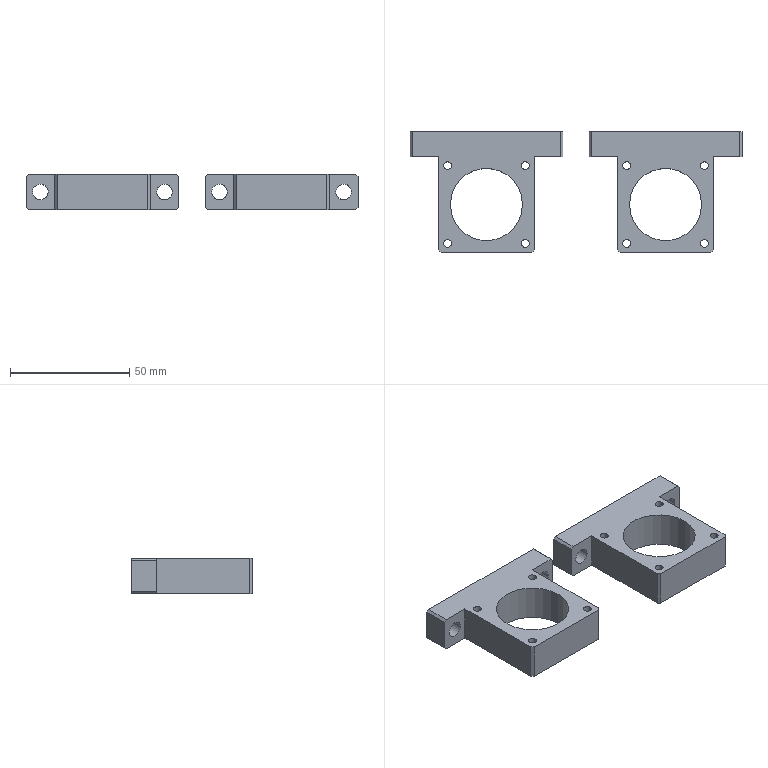Part | 2 solids | 46 faces | box 139 x 50.5 x 15 mm | volume 44135 mm3 | plane 32 | cylinder 14 | commonest cylinder face diameters 3.3 x8 6.6 x4 30.2 x2
STEP:
#1=CARTESIAN_POINT('',(94.,-25.25,7.5));
#2=VERTEX_POINT('',#1);
#3=CARTESIAN_POINT('',(95.,-24.25,7.5));
#4=VERTEX_POINT('',#3);
#5=CARTESIAN_POINT('',(95.,-24.25,7.5));
#6=DIRECTION('',(0.7071,0.7071,0.));
#7=VECTOR('',#6,1000.);
#8=LINE('',#5,#7);
#9=EDGE_CURVE('',#2,#4,#8,.T.);
#10=ORIENTED_EDGE('',*,*,#9,.F.);
#11=CARTESIAN_POINT('',(94.,-25.25,-7.5));
#12=VERTEX_POINT('',#11);
#13=CARTESIAN_POINT('',(94.,-25.25,7.5));
#14=DIRECTION('',(0.,0.,1.));
#15=VECTOR('',#14,1000.);
#16=LINE('',#13,#15);
#17=EDGE_CURVE('',#12,#2,#16,.T.);
#18=ORIENTED_EDGE('',*,*,#17,.F.);
#19=CARTESIAN_POINT('',(95.,-24.25,-7.5));
#20=VERTEX_POINT('',#19);
#21=CARTESIAN_POINT('',(97.125,-22.125,-7.5));
#22=DIRECTION('',(-0.7071,-0.7071,0.));
#23=VECTOR('',#22,1000.);
#24=LINE('',#21,#23);
#25=EDGE_CURVE('',#20,#12,#24,.T.);
#26=ORIENTED_EDGE('',*,*,#25,.F.);
#27=CARTESIAN_POINT('',(95.,-24.25,-7.5));
#28=DIRECTION('',(0.,0.,-1.));
#29=VECTOR('',#28,1000.);
#30=LINE('',#27,#29);
#31=EDGE_CURVE('',#4,#20,#30,.T.);
#32=ORIENTED_EDGE('',*,*,#31,.F.);
#33=EDGE_LOOP('',(#10,#18,#26,#32));
#34=FACE_BOUND('',#33,.T.);
#35=CARTESIAN_POINT('',(95.,-24.25,7.5));
#36=DIRECTION('',(0.7071,-0.7071,0.));
#37=DIRECTION('',(0.,0.,1.));
#38=AXIS2_PLACEMENT_3D('',#35,#36,#37);
#39=PLANE('',#38);
#40=ADVANCED_FACE('',(#34),#39,.T.);
#41=CARTESIAN_POINT('',(55.,-24.25,7.5));
#42=VERTEX_POINT('',#41);
#43=CARTESIAN_POINT('',(56.,-25.25,7.5));
#44=VERTEX_POINT('',#43);
#45=CARTESIAN_POINT('',(56.,-25.25,7.5));
#46=DIRECTION('',(0.7071,-0.7071,0.));
#47=VECTOR('',#46,1000.);
#48=LINE('',#45,#47);
#49=EDGE_CURVE('',#42,#44,#48,.T.);
#50=ORIENTED_EDGE('',*,*,#49,.F.);
#51=CARTESIAN_POINT('',(55.,-24.25,-7.5));
#52=VERTEX_POINT('',#51);
#53=CARTESIAN_POINT('',(55.,-24.25,7.5));
#54=DIRECTION('',(0.,0.,1.));
#55=VECTOR('',#54,1000.);
#56=LINE('',#53,#55);
#57=EDGE_CURVE('',#52,#42,#56,.T.);
#58=ORIENTED_EDGE('',*,*,#57,.F.);
#59=CARTESIAN_POINT('',(56.,-25.25,-7.5));
#60=VERTEX_POINT('',#59);
#61=CARTESIAN_POINT('',(52.875,-22.125,-7.5));
#62=DIRECTION('',(-0.7071,0.7071,0.));
#63=VECTOR('',#62,1000.);
#64=LINE('',#61,#63);
#65=EDGE_CURVE('',#60,#52,#64,.T.);
#66=ORIENTED_EDGE('',*,*,#65,.F.);
#67=CARTESIAN_POINT('',(56.,-25.25,-7.5));
#68=DIRECTION('',(0.,0.,-1.));
#69=VECTOR('',#68,1000.);
#70=LINE('',#67,#69);
#71=EDGE_CURVE('',#44,#60,#70,.T.);
#72=ORIENTED_EDGE('',*,*,#71,.F.);
#73=EDGE_LOOP('',(#50,#58,#66,#72));
#74=FACE_BOUND('',#73,.T.);
#75=CARTESIAN_POINT('',(56.,-25.25,7.5));
#76=DIRECTION('',(-0.7071,-0.7071,0.));
#77=DIRECTION('',(0.,0.,1.));
#78=AXIS2_PLACEMENT_3D('',#75,#76,#77);
#79=PLANE('',#78);
#80=ADVANCED_FACE('',(#74),#79,.T.);
#81=CARTESIAN_POINT('',(44.,14.75,7.5));
#82=VERTEX_POINT('',#81);
#83=CARTESIAN_POINT('',(43.,14.75,6.5));
#84=VERTEX_POINT('',#83);
#85=CARTESIAN_POINT('',(43.5,14.75,7.));
#86=DIRECTION('',(-0.7071,0.,-0.7071));
#87=VECTOR('',#86,1000.);
#88=LINE('',#85,#87);
#89=EDGE_CURVE('',#82,#84,#88,.T.);
#90=ORIENTED_EDGE('',*,*,#89,.F.);
#91=CARTESIAN_POINT('',(44.,25.25,7.5));
#92=VERTEX_POINT('',#91);
#93=CARTESIAN_POINT('',(44.,14.75,7.5));
#94=DIRECTION('',(0.,-1.,0.));
#95=VECTOR('',#94,1000.);
#96=LINE('',#93,#95);
#97=EDGE_CURVE('',#92,#82,#96,.T.);
#98=ORIENTED_EDGE('',*,*,#97,.F.);
#99=CARTESIAN_POINT('',(43.,25.25,6.5));
#100=VERTEX_POINT('',#99);
#101=CARTESIAN_POINT('',(43.5,25.25,7.));
#102=DIRECTION('',(0.7071,0.,0.7071));
#103=VECTOR('',#102,1000.);
#104=LINE('',#101,#103);
#105=EDGE_CURVE('',#100,#92,#104,.T.);
#106=ORIENTED_EDGE('',*,*,#105,.F.);
#107=CARTESIAN_POINT('',(43.,25.25,6.5));
#108=DIRECTION('',(0.,1.,0.));
#109=VECTOR('',#108,1000.);
#110=LINE('',#107,#109);
#111=EDGE_CURVE('',#84,#100,#110,.T.);
#112=ORIENTED_EDGE('',*,*,#111,.F.);
#113=EDGE_LOOP('',(#90,#98,#106,#112));
#114=FACE_BOUND('',#113,.T.);
#115=CARTESIAN_POINT('',(43.,-25.25,6.5));
#116=DIRECTION('',(-0.7071,0.,0.7071));
#117=DIRECTION('',(0.,-1.,0.));
#118=AXIS2_PLACEMENT_3D('',#115,#116,#117);
#119=PLANE('',#118);
#120=ADVANCED_FACE('',(#114),#119,.T.);
#121=CARTESIAN_POINT('',(43.,14.75,-6.5));
#122=VERTEX_POINT('',#121);
#123=CARTESIAN_POINT('',(44.,14.75,-7.5));
#124=VERTEX_POINT('',#123);
#125=CARTESIAN_POINT('',(36.,14.75,0.5));
#126=DIRECTION('',(0.7071,0.,-0.7071));
#127=VECTOR('',#126,1000.);
#128=LINE('',#125,#127);
#129=EDGE_CURVE('',#122,#124,#128,.T.);
#130=ORIENTED_EDGE('',*,*,#129,.F.);
#131=CARTESIAN_POINT('',(43.,25.25,-6.5));
#132=VERTEX_POINT('',#131);
#133=CARTESIAN_POINT('',(43.,-25.25,-6.5));
#134=DIRECTION('',(0.,-1.,0.));
#135=VECTOR('',#134,1000.);
#136=LINE('',#133,#135);
#137=EDGE_CURVE('',#132,#122,#136,.T.);
#138=ORIENTED_EDGE('',*,*,#137,.F.);
#139=CARTESIAN_POINT('',(44.,25.25,-7.5));
#140=VERTEX_POINT('',#139);
#141=CARTESIAN_POINT('',(36.,25.25,0.5));
#142=DIRECTION('',(-0.7071,0.,0.7071));
#143=VECTOR('',#142,1000.);
#144=LINE('',#141,#143);
#145=EDGE_CURVE('',#140,#132,#144,.T.);
#146=ORIENTED_EDGE('',*,*,#145,.F.);
#147=CARTESIAN_POINT('',(44.,0.,-7.5));
#148=DIRECTION('',(0.,1.,0.));
#149=VECTOR('',#148,1000.);
#150=LINE('',#147,#149);
#151=EDGE_CURVE('',#124,#140,#150,.T.);
#152=ORIENTED_EDGE('',*,*,#151,.F.);
#153=EDGE_LOOP('',(#130,#138,#146,#152));
#154=FACE_BOUND('',#153,.T.);
#155=CARTESIAN_POINT('',(44.,0.,-7.5));
#156=DIRECTION('',(0.7071,0.,0.7071));
#157=DIRECTION('',(0.,1.,0.));
#158=AXIS2_PLACEMENT_3D('',#155,#156,#157);
#159=PLANE('',#158);
#160=ADVANCED_FACE('',(#154),#159,.F.);
#161=CARTESIAN_POINT('',(107.,14.75,6.5));
#162=VERTEX_POINT('',#161);
#163=CARTESIAN_POINT('',(106.,14.75,7.5));
#164=VERTEX_POINT('',#163);
#165=CARTESIAN_POINT('',(74.5,14.75,39.));
#166=DIRECTION('',(-0.7071,0.,0.7071));
#167=VECTOR('',#166,1000.);
#168=LINE('',#165,#167);
#169=EDGE_CURVE('',#162,#164,#168,.T.);
#170=ORIENTED_EDGE('',*,*,#169,.F.);
#171=CARTESIAN_POINT('',(107.,25.25,6.5));
#172=VERTEX_POINT('',#171);
#173=CARTESIAN_POINT('',(107.,-25.25,6.5));
#174=DIRECTION('',(0.,-1.,0.));
#175=VECTOR('',#174,1000.);
#176=LINE('',#173,#175);
#177=EDGE_CURVE('',#172,#162,#176,.T.);
#178=ORIENTED_EDGE('',*,*,#177,.F.);
#179=CARTESIAN_POINT('',(106.,25.25,7.5));
#180=VERTEX_POINT('',#179);
#181=CARTESIAN_POINT('',(74.5,25.25,39.));
#182=DIRECTION('',(0.7071,0.,-0.7071));
#183=VECTOR('',#182,1000.);
#184=LINE('',#181,#183);
#185=EDGE_CURVE('',#180,#172,#184,.T.);
#186=ORIENTED_EDGE('',*,*,#185,.F.);
#187=CARTESIAN_POINT('',(106.,0.,7.5));
#188=DIRECTION('',(0.,1.,0.));
#189=VECTOR('',#188,1000.);
#190=LINE('',#187,#189);
#191=EDGE_CURVE('',#164,#180,#190,.T.);
#192=ORIENTED_EDGE('',*,*,#191,.F.);
#193=EDGE_LOOP('',(#170,#178,#186,#192));
#194=FACE_BOUND('',#193,.T.);
#195=CARTESIAN_POINT('',(106.,0.,7.5));
#196=DIRECTION('',(-0.7071,0.,-0.7071));
#197=DIRECTION('',(0.,1.,0.));
#198=AXIS2_PLACEMENT_3D('',#195,#196,#197);
#199=PLANE('',#198);
#200=ADVANCED_FACE('',(#194),#199,.F.);
#201=CARTESIAN_POINT('',(106.,14.75,-7.5));
#202=VERTEX_POINT('',#201);
#203=CARTESIAN_POINT('',(107.,14.75,-6.5));
#204=VERTEX_POINT('',#203);
#205=CARTESIAN_POINT('',(82.,14.75,-31.5));
#206=DIRECTION('',(0.7071,0.,0.7071));
#207=VECTOR('',#206,1000.);
#208=LINE('',#205,#207);
#209=EDGE_CURVE('',#202,#204,#208,.T.);
#210=ORIENTED_EDGE('',*,*,#209,.F.);
#211=CARTESIAN_POINT('',(106.,25.25,-7.5));
#212=VERTEX_POINT('',#211);
#213=CARTESIAN_POINT('',(106.,14.75,-7.5));
#214=DIRECTION('',(0.,-1.,0.));
#215=VECTOR('',#214,1000.);
#216=LINE('',#213,#215);
#217=EDGE_CURVE('',#212,#202,#216,.T.);
#218=ORIENTED_EDGE('',*,*,#217,.F.);
#219=CARTESIAN_POINT('',(107.,25.25,-6.5));
#220=VERTEX_POINT('',#219);
#221=CARTESIAN_POINT('',(82.,25.25,-31.5));
#222=DIRECTION('',(-0.7071,0.,-0.7071));
#223=VECTOR('',#222,1000.);
#224=LINE('',#221,#223);
#225=EDGE_CURVE('',#220,#212,#224,.T.);
#226=ORIENTED_EDGE('',*,*,#225,.F.);
#227=CARTESIAN_POINT('',(107.,25.25,-6.5));
#228=DIRECTION('',(0.,1.,0.));
#229=VECTOR('',#228,1000.);
#230=LINE('',#227,#229);
#231=EDGE_CURVE('',#204,#220,#230,.T.);
#232=ORIENTED_EDGE('',*,*,#231,.F.);
#233=EDGE_LOOP('',(#210,#218,#226,#232));
#234=FACE_BOUND('',#233,.T.);
#235=CARTESIAN_POINT('',(107.,-25.25,-6.5));
#236=DIRECTION('',(0.7071,0.,-0.7071));
#237=DIRECTION('',(0.,-1.,0.));
#238=AXIS2_PLACEMENT_3D('',#235,#236,#237);
#239=PLANE('',#238);
#240=ADVANCED_FACE('',(#234),#239,.T.);
#241=CARTESIAN_POINT('',(43.,14.75,7.5));
#242=DIRECTION('',(0.,0.,-1.));
#243=VECTOR('',#242,1000.);
#244=LINE('',#241,#243);
#245=EDGE_CURVE('',#84,#122,#244,.T.);
#246=ORIENTED_EDGE('',*,*,#245,.T.);
#247=ORIENTED_EDGE('',*,*,#129,.T.);
#248=CARTESIAN_POINT('',(55.,14.75,-7.5));
#249=VERTEX_POINT('',#248);
#250=CARTESIAN_POINT('',(43.,14.75,-7.5));
#251=DIRECTION('',(-1.,0.,0.));
#252=VECTOR('',#251,1000.);
#253=LINE('',#250,#252);
#254=EDGE_CURVE('',#249,#124,#253,.T.);
#255=ORIENTED_EDGE('',*,*,#254,.F.);
#256=CARTESIAN_POINT('',(55.,14.75,7.5));
#257=VERTEX_POINT('',#256);
#258=CARTESIAN_POINT('',(55.,14.75,7.5));
#259=DIRECTION('',(0.,0.,-1.));
#260=VECTOR('',#259,1000.);
#261=LINE('',#258,#260);
#262=EDGE_CURVE('',#257,#249,#261,.T.);
#263=ORIENTED_EDGE('',*,*,#262,.F.);
#264=CARTESIAN_POINT('',(43.,14.75,7.5));
#265=DIRECTION('',(-1.,0.,0.));
#266=VECTOR('',#265,1000.);
#267=LINE('',#264,#266);
#268=EDGE_CURVE('',#257,#82,#267,.T.);
#269=ORIENTED_EDGE('',*,*,#268,.T.);
#270=ORIENTED_EDGE('',*,*,#89,.T.);
#271=EDGE_LOOP('',(#246,#247,#255,#263,#269,#270));
#272=FACE_BOUND('',#271,.T.);
#273=CARTESIAN_POINT('',(52.3,14.75,0.));
#274=VERTEX_POINT('',#273);
#275=CARTESIAN_POINT('',(49.,14.75,0.));
#276=DIRECTION('',(0.,-1.,0.));
#277=DIRECTION('',(1.,0.,0.));
#278=AXIS2_PLACEMENT_3D('',#275,#276,#277);
#279=CIRCLE('',#278,3.3);
#280=EDGE_CURVE('',#274,#274,#279,.T.);
#281=ORIENTED_EDGE('',*,*,#280,.F.);
#282=EDGE_LOOP('',(#281));
#283=FACE_BOUND('',#282,.T.);
#284=CARTESIAN_POINT('',(43.,14.75,7.5));
#285=DIRECTION('',(0.,-1.,0.));
#286=DIRECTION('',(1.,0.,0.));
#287=AXIS2_PLACEMENT_3D('',#284,#285,#286);
#288=PLANE('',#287);
#289=ADVANCED_FACE('',(#272,#283),#288,.T.);
#290=CARTESIAN_POINT('',(55.,-25.25,-7.5));
#291=DIRECTION('',(0.,1.,0.));
#292=VECTOR('',#291,1000.);
#293=LINE('',#290,#292);
#294=EDGE_CURVE('',#52,#249,#293,.T.);
#295=ORIENTED_EDGE('',*,*,#294,.F.);
#296=ORIENTED_EDGE('',*,*,#57,.T.);
#297=CARTESIAN_POINT('',(55.,-25.25,7.5));
#298=DIRECTION('',(0.,1.,0.));
#299=VECTOR('',#298,1000.);
#300=LINE('',#297,#299);
#301=EDGE_CURVE('',#42,#257,#300,.T.);
#302=ORIENTED_EDGE('',*,*,#301,.T.);
#303=ORIENTED_EDGE('',*,*,#262,.T.);
#304=EDGE_LOOP('',(#295,#296,#302,#303));
#305=FACE_BOUND('',#304,.T.);
#306=CARTESIAN_POINT('',(55.,-25.25,7.5));
#307=DIRECTION('',(-1.,0.,0.));
#308=DIRECTION('',(0.,-1.,0.));
#309=AXIS2_PLACEMENT_3D('',#306,#307,#308);
#310=PLANE('',#309);
#311=ADVANCED_FACE('',(#305),#310,.T.);
#312=CARTESIAN_POINT('',(95.,14.75,7.5));
#313=VERTEX_POINT('',#312);
#314=CARTESIAN_POINT('',(95.,-25.25,7.5));
#315=DIRECTION('',(0.,-1.,0.));
#316=VECTOR('',#315,1000.);
#317=LINE('',#314,#316);
#318=EDGE_CURVE('',#313,#4,#317,.T.);
#319=ORIENTED_EDGE('',*,*,#318,.T.);
#320=ORIENTED_EDGE('',*,*,#31,.T.);
#321=CARTESIAN_POINT('',(95.,14.75,-7.5));
#322=VERTEX_POINT('',#321);
#323=CARTESIAN_POINT('',(95.,-25.25,-7.5));
#324=DIRECTION('',(0.,-1.,0.));
#325=VECTOR('',#324,1000.);
#326=LINE('',#323,#325);
#327=EDGE_CURVE('',#322,#20,#326,.T.);
#328=ORIENTED_EDGE('',*,*,#327,.F.);
#329=CARTESIAN_POINT('',(95.,14.75,7.5));
#330=DIRECTION('',(0.,0.,-1.));
#331=VECTOR('',#330,1000.);
#332=LINE('',#329,#331);
#333=EDGE_CURVE('',#313,#322,#332,.T.);
#334=ORIENTED_EDGE('',*,*,#333,.F.);
#335=EDGE_LOOP('',(#319,#320,#328,#334));
#336=FACE_BOUND('',#335,.T.);
#337=CARTESIAN_POINT('',(95.,-25.25,7.5));
#338=DIRECTION('',(1.,0.,0.));
#339=DIRECTION('',(0.,1.,0.));
#340=AXIS2_PLACEMENT_3D('',#337,#338,#339);
#341=PLANE('',#340);
#342=ADVANCED_FACE('',(#336),#341,.T.);
#343=CARTESIAN_POINT('',(75.,14.75,-7.5));
#344=DIRECTION('',(-1.,0.,0.));
#345=VECTOR('',#344,1000.);
#346=LINE('',#343,#345);
#347=EDGE_CURVE('',#202,#322,#346,.T.);
#348=ORIENTED_EDGE('',*,*,#347,.F.);
#349=ORIENTED_EDGE('',*,*,#209,.T.);
#350=CARTESIAN_POINT('',(107.,14.75,7.5));
#351=DIRECTION('',(0.,0.,-1.));
#352=VECTOR('',#351,1000.);
#353=LINE('',#350,#352);
#354=EDGE_CURVE('',#162,#204,#353,.T.);
#355=ORIENTED_EDGE('',*,*,#354,.F.);
#356=ORIENTED_EDGE('',*,*,#169,.T.);
#357=CARTESIAN_POINT('',(43.,14.75,7.5));
#358=DIRECTION('',(-1.,0.,0.));
#359=VECTOR('',#358,1000.);
#360=LINE('',#357,#359);
#361=EDGE_CURVE('',#164,#313,#360,.T.);
#362=ORIENTED_EDGE('',*,*,#361,.T.);
#363=ORIENTED_EDGE('',*,*,#333,.T.);
#364=EDGE_LOOP('',(#348,#349,#355,#356,#362,#363));
#365=FACE_BOUND('',#364,.T.);
#366=CARTESIAN_POINT('',(104.3,14.75,0.));
#367=VERTEX_POINT('',#366);
#368=CARTESIAN_POINT('',(101.,14.75,0.));
#369=DIRECTION('',(0.,-1.,0.));
#370=DIRECTION('',(1.,0.,0.));
#371=AXIS2_PLACEMENT_3D('',#368,#369,#370);
#372=CIRCLE('',#371,3.3);
#373=EDGE_CURVE('',#367,#367,#372,.T.);
#374=ORIENTED_EDGE('',*,*,#373,.F.);
#375=EDGE_LOOP('',(#374));
#376=FACE_BOUND('',#375,.T.);
#377=CARTESIAN_POINT('',(43.,14.75,7.5));
#378=DIRECTION('',(0.,-1.,0.));
#379=DIRECTION('',(1.,0.,0.));
#380=AXIS2_PLACEMENT_3D('',#377,#378,#379);
#381=PLANE('',#380);
#382=ADVANCED_FACE('',(#365,#376),#381,.T.);
#383=CARTESIAN_POINT('',(107.,25.25,7.5));
#384=DIRECTION('',(0.,0.,-1.));
#385=VECTOR('',#384,1000.);
#386=LINE('',#383,#385);
#387=EDGE_CURVE('',#172,#220,#386,.T.);
#388=ORIENTED_EDGE('',*,*,#387,.T.);
#389=ORIENTED_EDGE('',*,*,#225,.T.);
#390=CARTESIAN_POINT('',(43.,25.25,-7.5));
#391=DIRECTION('',(1.,0.,0.));
#392=VECTOR('',#391,1000.);
#393=LINE('',#390,#392);
#394=EDGE_CURVE('',#140,#212,#393,.T.);
#395=ORIENTED_EDGE('',*,*,#394,.F.);
#396=ORIENTED_EDGE('',*,*,#145,.T.);
#397=CARTESIAN_POINT('',(43.,25.25,7.5));
#398=DIRECTION('',(0.,0.,-1.));
#399=VECTOR('',#398,1000.);
#400=LINE('',#397,#399);
#401=EDGE_CURVE('',#100,#132,#400,.T.);
#402=ORIENTED_EDGE('',*,*,#401,.F.);
#403=ORIENTED_EDGE('',*,*,#105,.T.);
#404=CARTESIAN_POINT('',(43.,25.25,7.5));
#405=DIRECTION('',(1.,0.,0.));
#406=VECTOR('',#405,1000.);
#407=LINE('',#404,#406);
#408=EDGE_CURVE('',#92,#180,#407,.T.);
#409=ORIENTED_EDGE('',*,*,#408,.T.);
#410=ORIENTED_EDGE('',*,*,#185,.T.);
#411=EDGE_LOOP('',(#388,#389,#395,#396,#402,#403,#409,#410));
#412=FACE_BOUND('',#411,.T.);
#413=CARTESIAN_POINT('',(101.,25.25,3.3));
#414=VERTEX_POINT('',#413);
#415=CARTESIAN_POINT('',(101.,25.25,0.));
#416=DIRECTION('',(0.,1.,0.));
#417=DIRECTION('',(0.,0.,1.));
#418=AXIS2_PLACEMENT_3D('',#415,#416,#417);
#419=CIRCLE('',#418,3.3);
#420=EDGE_CURVE('',#414,#414,#419,.T.);
#421=ORIENTED_EDGE('',*,*,#420,.F.);
#422=EDGE_LOOP('',(#421));
#423=FACE_BOUND('',#422,.T.);
#424=CARTESIAN_POINT('',(49.,25.25,3.3));
#425=VERTEX_POINT('',#424);
#426=CARTESIAN_POINT('',(49.,25.25,0.));
#427=DIRECTION('',(0.,1.,0.));
#428=DIRECTION('',(0.,0.,1.));
#429=AXIS2_PLACEMENT_3D('',#426,#427,#428);
#430=CIRCLE('',#429,3.3);
#431=EDGE_CURVE('',#425,#425,#430,.T.);
#432=ORIENTED_EDGE('',*,*,#431,.F.);
#433=EDGE_LOOP('',(#432));
#434=FACE_BOUND('',#433,.T.);
#435=CARTESIAN_POINT('',(43.,25.25,7.5));
#436=DIRECTION('',(0.,1.,0.));
#437=DIRECTION('',(0.,0.,1.));
#438=AXIS2_PLACEMENT_3D('',#435,#436,#437);
#439=PLANE('',#438);
#440=ADVANCED_FACE('',(#412,#423,#434),#439,.T.);
#441=ORIENTED_EDGE('',*,*,#394,.T.);
#442=ORIENTED_EDGE('',*,*,#217,.T.);
#443=ORIENTED_EDGE('',*,*,#347,.T.);
#444=ORIENTED_EDGE('',*,*,#327,.T.);
#445=ORIENTED_EDGE('',*,*,#25,.T.);
#446=CARTESIAN_POINT('',(43.,-25.25,-7.5));
#447=DIRECTION('',(1.,0.,0.));
#448=VECTOR('',#447,1000.);
#449=LINE('',#446,#448);
#450=EDGE_CURVE('',#60,#12,#449,.T.);
#451=ORIENTED_EDGE('',*,*,#450,.F.);
#452=ORIENTED_EDGE('',*,*,#65,.T.);
#453=ORIENTED_EDGE('',*,*,#294,.T.);
#454=ORIENTED_EDGE('',*,*,#254,.T.);
#455=ORIENTED_EDGE('',*,*,#151,.T.);
#456=EDGE_LOOP('',(#441,#442,#443,#444,#445,#451,#452,#453,#454,#455));
#457=FACE_BOUND('',#456,.T.);
#458=CARTESIAN_POINT('',(59.9,-5.25,-7.5));
#459=VERTEX_POINT('',#458);
#460=CARTESIAN_POINT('',(75.,-5.25,-7.5));
#461=DIRECTION('',(0.,0.,-1.));
#462=DIRECTION('',(-1.,0.,0.));
#463=AXIS2_PLACEMENT_3D('',#460,#461,#462);
#464=CIRCLE('',#463,15.1);
#465=EDGE_CURVE('',#459,#459,#464,.T.);
#466=ORIENTED_EDGE('',*,*,#465,.F.);
#467=EDGE_LOOP('',(#466));
#468=FACE_BOUND('',#467,.T.);
#469=CARTESIAN_POINT('',(57.087,11.013,-7.5));
#470=VERTEX_POINT('',#469);
#471=CARTESIAN_POINT('',(58.737,11.013,-7.5));
#472=DIRECTION('',(0.,0.,-1.));
#473=DIRECTION('',(-1.,0.,0.));
#474=AXIS2_PLACEMENT_3D('',#471,#472,#473);
#475=CIRCLE('',#474,1.65);
#476=EDGE_CURVE('',#470,#470,#475,.T.);
#477=ORIENTED_EDGE('',*,*,#476,.F.);
#478=EDGE_LOOP('',(#477));
#479=FACE_BOUND('',#478,.T.);
#480=CARTESIAN_POINT('',(89.613,11.013,-7.5));
#481=VERTEX_POINT('',#480);
#482=CARTESIAN_POINT('',(91.263,11.013,-7.5));
#483=DIRECTION('',(0.,0.,-1.));
#484=DIRECTION('',(-1.,0.,0.));
#485=AXIS2_PLACEMENT_3D('',#482,#483,#484);
#486=CIRCLE('',#485,1.65);
#487=EDGE_CURVE('',#481,#481,#486,.T.);
#488=ORIENTED_EDGE('',*,*,#487,.F.);
#489=EDGE_LOOP('',(#488));
#490=FACE_BOUND('',#489,.T.);
#491=CARTESIAN_POINT('',(89.613,-21.513,-7.5));
#492=VERTEX_POINT('',#491);
#493=CARTESIAN_POINT('',(91.263,-21.513,-7.5));
#494=DIRECTION('',(0.,0.,-1.));
#495=DIRECTION('',(-1.,0.,0.));
#496=AXIS2_PLACEMENT_3D('',#493,#494,#495);
#497=CIRCLE('',#496,1.65);
#498=EDGE_CURVE('',#492,#492,#497,.T.);
#499=ORIENTED_EDGE('',*,*,#498,.F.);
#500=EDGE_LOOP('',(#499));
#501=FACE_BOUND('',#500,.T.);
#502=CARTESIAN_POINT('',(57.087,-21.513,-7.5));
#503=VERTEX_POINT('',#502);
#504=CARTESIAN_POINT('',(58.737,-21.513,-7.5));
#505=DIRECTION('',(0.,0.,-1.));
#506=DIRECTION('',(-1.,0.,0.));
#507=AXIS2_PLACEMENT_3D('',#504,#505,#506);
#508=CIRCLE('',#507,1.65);
#509=EDGE_CURVE('',#503,#503,#508,.T.);
#510=ORIENTED_EDGE('',*,*,#509,.F.);
#511=EDGE_LOOP('',(#510));
#512=FACE_BOUND('',#511,.T.);
#513=CARTESIAN_POINT('',(75.,0.,-7.5));
#514=DIRECTION('',(0.,0.,-1.));
#515=DIRECTION('',(-1.,0.,0.));
#516=AXIS2_PLACEMENT_3D('',#513,#514,#515);
#517=PLANE('',#516);
#518=ADVANCED_FACE('',(#457,#468,#479,#490,#501,#512),#517,.T.);
#519=ORIENTED_EDGE('',*,*,#361,.F.);
#520=ORIENTED_EDGE('',*,*,#191,.T.);
#521=ORIENTED_EDGE('',*,*,#408,.F.);
#522=ORIENTED_EDGE('',*,*,#97,.T.);
#523=ORIENTED_EDGE('',*,*,#268,.F.);
#524=ORIENTED_EDGE('',*,*,#301,.F.);
#525=ORIENTED_EDGE('',*,*,#49,.T.);
#526=CARTESIAN_POINT('',(43.,-25.25,7.5));
#527=DIRECTION('',(1.,0.,0.));
#528=VECTOR('',#527,1000.);
#529=LINE('',#526,#528);
#530=EDGE_CURVE('',#44,#2,#529,.T.);
#531=ORIENTED_EDGE('',*,*,#530,.T.);
#532=ORIENTED_EDGE('',*,*,#9,.T.);
#533=ORIENTED_EDGE('',*,*,#318,.F.);
#534=EDGE_LOOP('',(#519,#520,#521,#522,#523,#524,#525,#531,#532,#533));
#535=FACE_BOUND('',#534,.T.);
#536=CARTESIAN_POINT('',(59.9,-5.25,7.5));
#537=VERTEX_POINT('',#536);
#538=CARTESIAN_POINT('',(75.,-5.25,7.5));
#539=DIRECTION('',(0.,0.,-1.));
#540=DIRECTION('',(-1.,0.,0.));
#541=AXIS2_PLACEMENT_3D('',#538,#539,#540);
#542=CIRCLE('',#541,15.1);
#543=EDGE_CURVE('',#537,#537,#542,.T.);
#544=ORIENTED_EDGE('',*,*,#543,.T.);
#545=EDGE_LOOP('',(#544));
#546=FACE_BOUND('',#545,.T.);
#547=CARTESIAN_POINT('',(57.087,11.013,7.5));
#548=VERTEX_POINT('',#547);
#549=CARTESIAN_POINT('',(58.737,11.013,7.5));
#550=DIRECTION('',(0.,0.,-1.));
#551=DIRECTION('',(-1.,0.,0.));
#552=AXIS2_PLACEMENT_3D('',#549,#550,#551);
#553=CIRCLE('',#552,1.65);
#554=EDGE_CURVE('',#548,#548,#553,.T.);
#555=ORIENTED_EDGE('',*,*,#554,.T.);
#556=EDGE_LOOP('',(#555));
#557=FACE_BOUND('',#556,.T.);
#558=CARTESIAN_POINT('',(89.613,11.013,7.5));
#559=VERTEX_POINT('',#558);
#560=CARTESIAN_POINT('',(91.263,11.013,7.5));
#561=DIRECTION('',(0.,0.,-1.));
#562=DIRECTION('',(-1.,0.,0.));
#563=AXIS2_PLACEMENT_3D('',#560,#561,#562);
#564=CIRCLE('',#563,1.65);
#565=EDGE_CURVE('',#559,#559,#564,.T.);
#566=ORIENTED_EDGE('',*,*,#565,.T.);
#567=EDGE_LOOP('',(#566));
#568=FACE_BOUND('',#567,.T.);
#569=CARTESIAN_POINT('',(89.613,-21.513,7.5));
#570=VERTEX_POINT('',#569);
#571=CARTESIAN_POINT('',(91.263,-21.513,7.5));
#572=DIRECTION('',(0.,0.,-1.));
#573=DIRECTION('',(-1.,0.,0.));
#574=AXIS2_PLACEMENT_3D('',#571,#572,#573);
#575=CIRCLE('',#574,1.65);
#576=EDGE_CURVE('',#570,#570,#575,.T.);
#577=ORIENTED_EDGE('',*,*,#576,.T.);
#578=EDGE_LOOP('',(#577));
#579=FACE_BOUND('',#578,.T.);
#580=CARTESIAN_POINT('',(57.087,-21.513,7.5));
#581=VERTEX_POINT('',#580);
#582=CARTESIAN_POINT('',(58.737,-21.513,7.5));
#583=DIRECTION('',(0.,0.,-1.));
#584=DIRECTION('',(-1.,0.,0.));
#585=AXIS2_PLACEMENT_3D('',#582,#583,#584);
#586=CIRCLE('',#585,1.65);
#587=EDGE_CURVE('',#581,#581,#586,.T.);
#588=ORIENTED_EDGE('',*,*,#587,.T.);
#589=EDGE_LOOP('',(#588));
#590=FACE_BOUND('',#589,.T.);
#591=CARTESIAN_POINT('',(75.,0.,7.5));
#592=DIRECTION('',(0.,0.,-1.));
#593=DIRECTION('',(-1.,0.,0.));
#594=AXIS2_PLACEMENT_3D('',#591,#592,#593);
#595=PLANE('',#594);
#596=ADVANCED_FACE('',(#535,#546,#557,#568,#579,#590),#595,.F.);
#597=ORIENTED_EDGE('',*,*,#354,.T.);
#598=ORIENTED_EDGE('',*,*,#231,.T.);
#599=ORIENTED_EDGE('',*,*,#387,.F.);
#600=ORIENTED_EDGE('',*,*,#177,.T.);
#601=EDGE_LOOP('',(#597,#598,#599,#600));
#602=FACE_BOUND('',#601,.T.);
#603=CARTESIAN_POINT('',(107.,-25.25,7.5));
#604=DIRECTION('',(-1.,0.,0.));
#605=DIRECTION('',(0.,0.,1.));
#606=AXIS2_PLACEMENT_3D('',#603,#604,#605);
#607=PLANE('',#606);
#608=ADVANCED_FACE('',(#602),#607,.F.);
#609=ORIENTED_EDGE('',*,*,#530,.F.);
#610=ORIENTED_EDGE('',*,*,#71,.T.);
#611=ORIENTED_EDGE('',*,*,#450,.T.);
#612=ORIENTED_EDGE('',*,*,#17,.T.);
#613=EDGE_LOOP('',(#609,#610,#611,#612));
#614=FACE_BOUND('',#613,.T.);
#615=CARTESIAN_POINT('',(43.,-25.25,7.5));
#616=DIRECTION('',(0.,1.,0.));
#617=DIRECTION('',(0.,0.,1.));
#618=AXIS2_PLACEMENT_3D('',#615,#616,#617);
#619=PLANE('',#618);
#620=ADVANCED_FACE('',(#614),#619,.F.);
#621=ORIENTED_EDGE('',*,*,#401,.T.);
#622=ORIENTED_EDGE('',*,*,#137,.T.);
#623=ORIENTED_EDGE('',*,*,#245,.F.);
#624=ORIENTED_EDGE('',*,*,#111,.T.);
#625=EDGE_LOOP('',(#621,#622,#623,#624));
#626=FACE_BOUND('',#625,.T.);
#627=CARTESIAN_POINT('',(43.,-25.25,7.5));
#628=DIRECTION('',(-1.,0.,0.));
#629=DIRECTION('',(0.,0.,1.));
#630=AXIS2_PLACEMENT_3D('',#627,#628,#629);
#631=PLANE('',#630);
#632=ADVANCED_FACE('',(#626),#631,.T.);
#633=ORIENTED_EDGE('',*,*,#465,.T.);
#634=EDGE_LOOP('',(#633));
#635=FACE_BOUND('',#634,.T.);
#636=ORIENTED_EDGE('',*,*,#543,.F.);
#637=EDGE_LOOP('',(#636));
#638=FACE_BOUND('',#637,.T.);
#639=CARTESIAN_POINT('',(75.,-5.25,7.5));
#640=DIRECTION('',(0.,0.,-1.));
#641=DIRECTION('',(-1.,0.,0.));
#642=AXIS2_PLACEMENT_3D('',#639,#640,#641);
#643=CYLINDRICAL_SURFACE('',#642,15.1);
#644=ADVANCED_FACE('',(#635,#638),#643,.F.);
#645=ORIENTED_EDGE('',*,*,#476,.T.);
#646=EDGE_LOOP('',(#645));
#647=FACE_BOUND('',#646,.T.);
#648=ORIENTED_EDGE('',*,*,#554,.F.);
#649=EDGE_LOOP('',(#648));
#650=FACE_BOUND('',#649,.T.);
#651=CARTESIAN_POINT('',(58.737,11.013,-7.5));
#652=DIRECTION('',(0.,0.,-1.));
#653=DIRECTION('',(-1.,0.,0.));
#654=AXIS2_PLACEMENT_3D('',#651,#652,#653);
#655=CYLINDRICAL_SURFACE('',#654,1.65);
#656=ADVANCED_FACE('',(#647,#650),#655,.F.);
#657=ORIENTED_EDGE('',*,*,#487,.T.);
#658=EDGE_LOOP('',(#657));
#659=FACE_BOUND('',#658,.T.);
#660=ORIENTED_EDGE('',*,*,#565,.F.);
#661=EDGE_LOOP('',(#660));
#662=FACE_BOUND('',#661,.T.);
#663=CARTESIAN_POINT('',(91.263,11.013,-7.5));
#664=DIRECTION('',(0.,0.,-1.));
#665=DIRECTION('',(-1.,0.,0.));
#666=AXIS2_PLACEMENT_3D('',#663,#664,#665);
#667=CYLINDRICAL_SURFACE('',#666,1.65);
#668=ADVANCED_FACE('',(#659,#662),#667,.F.);
#669=ORIENTED_EDGE('',*,*,#498,.T.);
#670=EDGE_LOOP('',(#669));
#671=FACE_BOUND('',#670,.T.);
#672=ORIENTED_EDGE('',*,*,#576,.F.);
#673=EDGE_LOOP('',(#672));
#674=FACE_BOUND('',#673,.T.);
#675=CARTESIAN_POINT('',(91.263,-21.513,-7.5));
#676=DIRECTION('',(0.,0.,-1.));
#677=DIRECTION('',(-1.,0.,0.));
#678=AXIS2_PLACEMENT_3D('',#675,#676,#677);
#679=CYLINDRICAL_SURFACE('',#678,1.65);
#680=ADVANCED_FACE('',(#671,#674),#679,.F.);
#681=ORIENTED_EDGE('',*,*,#509,.T.);
#682=EDGE_LOOP('',(#681));
#683=FACE_BOUND('',#682,.T.);
#684=ORIENTED_EDGE('',*,*,#587,.F.);
#685=EDGE_LOOP('',(#684));
#686=FACE_BOUND('',#685,.T.);
#687=CARTESIAN_POINT('',(58.737,-21.513,-7.5));
#688=DIRECTION('',(0.,0.,-1.));
#689=DIRECTION('',(-1.,0.,0.));
#690=AXIS2_PLACEMENT_3D('',#687,#688,#689);
#691=CYLINDRICAL_SURFACE('',#690,1.65);
#692=ADVANCED_FACE('',(#683,#686),#691,.F.);
#693=ORIENTED_EDGE('',*,*,#373,.T.);
#694=EDGE_LOOP('',(#693));
#695=FACE_BOUND('',#694,.T.);
#696=ORIENTED_EDGE('',*,*,#420,.T.);
#697=EDGE_LOOP('',(#696));
#698=FACE_BOUND('',#697,.T.);
#699=CARTESIAN_POINT('',(101.,25.25,0.));
#700=DIRECTION('',(0.,1.,0.));
#701=DIRECTION('',(0.,0.,1.));
#702=AXIS2_PLACEMENT_3D('',#699,#700,#701);
#703=CYLINDRICAL_SURFACE('',#702,3.3);
#704=ADVANCED_FACE('',(#695,#698),#703,.F.);
#705=ORIENTED_EDGE('',*,*,#280,.T.);
#706=EDGE_LOOP('',(#705));
#707=FACE_BOUND('',#706,.T.);
#708=ORIENTED_EDGE('',*,*,#431,.T.);
#709=EDGE_LOOP('',(#708));
#710=FACE_BOUND('',#709,.T.);
#711=CARTESIAN_POINT('',(49.,25.25,0.));
#712=DIRECTION('',(0.,1.,0.));
#713=DIRECTION('',(0.,0.,1.));
#714=AXIS2_PLACEMENT_3D('',#711,#712,#713);
#715=CYLINDRICAL_SURFACE('',#714,3.3);
#716=ADVANCED_FACE('',(#707,#710),#715,.F.);
#717=CLOSED_SHELL('',(#40,#80,#120,#160,#200,#240,#289,#311,#342,#382,#440,#518,#596,#608,#620,#632,#644,#656,#668,#680,#692,#704,#716));
#718=MANIFOLD_SOLID_BREP('',#717);
#719=CARTESIAN_POINT('',(19.,-25.25,7.5));
#720=VERTEX_POINT('',#719);
#721=CARTESIAN_POINT('',(20.,-24.25,7.5));
#722=VERTEX_POINT('',#721);
#723=CARTESIAN_POINT('',(20.,-24.25,7.5));
#724=DIRECTION('',(0.7071,0.7071,0.));
#725=VECTOR('',#724,1000.);
#726=LINE('',#723,#725);
#727=EDGE_CURVE('',#720,#722,#726,.T.);
#728=ORIENTED_EDGE('',*,*,#727,.F.);
#729=CARTESIAN_POINT('',(19.,-25.25,-7.5));
#730=VERTEX_POINT('',#729);
#731=CARTESIAN_POINT('',(19.,-25.25,7.5));
#732=DIRECTION('',(0.,0.,1.));
#733=VECTOR('',#732,1000.);
#734=LINE('',#731,#733);
#735=EDGE_CURVE('',#730,#720,#734,.T.);
#736=ORIENTED_EDGE('',*,*,#735,.F.);
#737=CARTESIAN_POINT('',(20.,-24.25,-7.5));
#738=VERTEX_POINT('',#737);
#739=CARTESIAN_POINT('',(22.125,-22.125,-7.5));
#740=DIRECTION('',(-0.7071,-0.7071,0.));
#741=VECTOR('',#740,1000.);
#742=LINE('',#739,#741);
#743=EDGE_CURVE('',#738,#730,#742,.T.);
#744=ORIENTED_EDGE('',*,*,#743,.F.);
#745=CARTESIAN_POINT('',(20.,-24.25,-7.5));
#746=DIRECTION('',(0.,0.,-1.));
#747=VECTOR('',#746,1000.);
#748=LINE('',#745,#747);
#749=EDGE_CURVE('',#722,#738,#748,.T.);
#750=ORIENTED_EDGE('',*,*,#749,.F.);
#751=EDGE_LOOP('',(#728,#736,#744,#750));
#752=FACE_BOUND('',#751,.T.);
#753=CARTESIAN_POINT('',(20.,-24.25,7.5));
#754=DIRECTION('',(0.7071,-0.7071,0.));
#755=DIRECTION('',(0.,0.,1.));
#756=AXIS2_PLACEMENT_3D('',#753,#754,#755);
#757=PLANE('',#756);
#758=ADVANCED_FACE('',(#752),#757,.T.);
#759=CARTESIAN_POINT('',(-20.,-24.25,7.5));
#760=VERTEX_POINT('',#759);
#761=CARTESIAN_POINT('',(-19.,-25.25,7.5));
#762=VERTEX_POINT('',#761);
#763=CARTESIAN_POINT('',(-19.,-25.25,7.5));
#764=DIRECTION('',(0.7071,-0.7071,0.));
#765=VECTOR('',#764,1000.);
#766=LINE('',#763,#765);
#767=EDGE_CURVE('',#760,#762,#766,.T.);
#768=ORIENTED_EDGE('',*,*,#767,.F.);
#769=CARTESIAN_POINT('',(-20.,-24.25,-7.5));
#770=VERTEX_POINT('',#769);
#771=CARTESIAN_POINT('',(-20.,-24.25,7.5));
#772=DIRECTION('',(0.,0.,1.));
#773=VECTOR('',#772,1000.);
#774=LINE('',#771,#773);
#775=EDGE_CURVE('',#770,#760,#774,.T.);
#776=ORIENTED_EDGE('',*,*,#775,.F.);
#777=CARTESIAN_POINT('',(-19.,-25.25,-7.5));
#778=VERTEX_POINT('',#777);
#779=CARTESIAN_POINT('',(-22.125,-22.125,-7.5));
#780=DIRECTION('',(-0.7071,0.7071,0.));
#781=VECTOR('',#780,1000.);
#782=LINE('',#779,#781);
#783=EDGE_CURVE('',#778,#770,#782,.T.);
#784=ORIENTED_EDGE('',*,*,#783,.F.);
#785=CARTESIAN_POINT('',(-19.,-25.25,-7.5));
#786=DIRECTION('',(0.,0.,-1.));
#787=VECTOR('',#786,1000.);
#788=LINE('',#785,#787);
#789=EDGE_CURVE('',#762,#778,#788,.T.);
#790=ORIENTED_EDGE('',*,*,#789,.F.);
#791=EDGE_LOOP('',(#768,#776,#784,#790));
#792=FACE_BOUND('',#791,.T.);
#793=CARTESIAN_POINT('',(-19.,-25.25,7.5));
#794=DIRECTION('',(-0.7071,-0.7071,0.));
#795=DIRECTION('',(0.,0.,1.));
#796=AXIS2_PLACEMENT_3D('',#793,#794,#795);
#797=PLANE('',#796);
#798=ADVANCED_FACE('',(#792),#797,.T.);
#799=CARTESIAN_POINT('',(-31.,14.75,7.5));
#800=VERTEX_POINT('',#799);
#801=CARTESIAN_POINT('',(-32.,14.75,6.5));
#802=VERTEX_POINT('',#801);
#803=CARTESIAN_POINT('',(-31.5,14.75,7.));
#804=DIRECTION('',(-0.7071,0.,-0.7071));
#805=VECTOR('',#804,1000.);
#806=LINE('',#803,#805);
#807=EDGE_CURVE('',#800,#802,#806,.T.);
#808=ORIENTED_EDGE('',*,*,#807,.F.);
#809=CARTESIAN_POINT('',(-31.,25.25,7.5));
#810=VERTEX_POINT('',#809);
#811=CARTESIAN_POINT('',(-31.,14.75,7.5));
#812=DIRECTION('',(0.,-1.,0.));
#813=VECTOR('',#812,1000.);
#814=LINE('',#811,#813);
#815=EDGE_CURVE('',#810,#800,#814,.T.);
#816=ORIENTED_EDGE('',*,*,#815,.F.);
#817=CARTESIAN_POINT('',(-32.,25.25,6.5));
#818=VERTEX_POINT('',#817);
#819=CARTESIAN_POINT('',(-31.5,25.25,7.));
#820=DIRECTION('',(0.7071,0.,0.7071));
#821=VECTOR('',#820,1000.);
#822=LINE('',#819,#821);
#823=EDGE_CURVE('',#818,#810,#822,.T.);
#824=ORIENTED_EDGE('',*,*,#823,.F.);
#825=CARTESIAN_POINT('',(-32.,25.25,6.5));
#826=DIRECTION('',(0.,1.,0.));
#827=VECTOR('',#826,1000.);
#828=LINE('',#825,#827);
#829=EDGE_CURVE('',#802,#818,#828,.T.);
#830=ORIENTED_EDGE('',*,*,#829,.F.);
#831=EDGE_LOOP('',(#808,#816,#824,#830));
#832=FACE_BOUND('',#831,.T.);
#833=CARTESIAN_POINT('',(-32.,-25.25,6.5));
#834=DIRECTION('',(-0.7071,0.,0.7071));
#835=DIRECTION('',(0.,-1.,0.));
#836=AXIS2_PLACEMENT_3D('',#833,#834,#835);
#837=PLANE('',#836);
#838=ADVANCED_FACE('',(#832),#837,.T.);
#839=CARTESIAN_POINT('',(-32.,14.75,-6.5));
#840=VERTEX_POINT('',#839);
#841=CARTESIAN_POINT('',(-31.,14.75,-7.5));
#842=VERTEX_POINT('',#841);
#843=CARTESIAN_POINT('',(-39.,14.75,0.5));
#844=DIRECTION('',(0.7071,0.,-0.7071));
#845=VECTOR('',#844,1000.);
#846=LINE('',#843,#845);
#847=EDGE_CURVE('',#840,#842,#846,.T.);
#848=ORIENTED_EDGE('',*,*,#847,.F.);
#849=CARTESIAN_POINT('',(-32.,25.25,-6.5));
#850=VERTEX_POINT('',#849);
#851=CARTESIAN_POINT('',(-32.,-25.25,-6.5));
#852=DIRECTION('',(0.,-1.,0.));
#853=VECTOR('',#852,1000.);
#854=LINE('',#851,#853);
#855=EDGE_CURVE('',#850,#840,#854,.T.);
#856=ORIENTED_EDGE('',*,*,#855,.F.);
#857=CARTESIAN_POINT('',(-31.,25.25,-7.5));
#858=VERTEX_POINT('',#857);
#859=CARTESIAN_POINT('',(-39.,25.25,0.5));
#860=DIRECTION('',(-0.7071,0.,0.7071));
#861=VECTOR('',#860,1000.);
#862=LINE('',#859,#861);
#863=EDGE_CURVE('',#858,#850,#862,.T.);
#864=ORIENTED_EDGE('',*,*,#863,.F.);
#865=CARTESIAN_POINT('',(-31.,0.,-7.5));
#866=DIRECTION('',(0.,1.,0.));
#867=VECTOR('',#866,1000.);
#868=LINE('',#865,#867);
#869=EDGE_CURVE('',#842,#858,#868,.T.);
#870=ORIENTED_EDGE('',*,*,#869,.F.);
#871=EDGE_LOOP('',(#848,#856,#864,#870));
#872=FACE_BOUND('',#871,.T.);
#873=CARTESIAN_POINT('',(-31.,0.,-7.5));
#874=DIRECTION('',(0.7071,0.,0.7071));
#875=DIRECTION('',(0.,1.,0.));
#876=AXIS2_PLACEMENT_3D('',#873,#874,#875);
#877=PLANE('',#876);
#878=ADVANCED_FACE('',(#872),#877,.F.);
#879=CARTESIAN_POINT('',(32.,14.75,6.5));
#880=VERTEX_POINT('',#879);
#881=CARTESIAN_POINT('',(31.,14.75,7.5));
#882=VERTEX_POINT('',#881);
#883=CARTESIAN_POINT('',(-0.5,14.75,39.));
#884=DIRECTION('',(-0.7071,0.,0.7071));
#885=VECTOR('',#884,1000.);
#886=LINE('',#883,#885);
#887=EDGE_CURVE('',#880,#882,#886,.T.);
#888=ORIENTED_EDGE('',*,*,#887,.F.);
#889=CARTESIAN_POINT('',(32.,25.25,6.5));
#890=VERTEX_POINT('',#889);
#891=CARTESIAN_POINT('',(32.,-25.25,6.5));
#892=DIRECTION('',(0.,-1.,0.));
#893=VECTOR('',#892,1000.);
#894=LINE('',#891,#893);
#895=EDGE_CURVE('',#890,#880,#894,.T.);
#896=ORIENTED_EDGE('',*,*,#895,.F.);
#897=CARTESIAN_POINT('',(31.,25.25,7.5));
#898=VERTEX_POINT('',#897);
#899=CARTESIAN_POINT('',(-0.5,25.25,39.));
#900=DIRECTION('',(0.7071,0.,-0.7071));
#901=VECTOR('',#900,1000.);
#902=LINE('',#899,#901);
#903=EDGE_CURVE('',#898,#890,#902,.T.);
#904=ORIENTED_EDGE('',*,*,#903,.F.);
#905=CARTESIAN_POINT('',(31.,0.,7.5));
#906=DIRECTION('',(0.,1.,0.));
#907=VECTOR('',#906,1000.);
#908=LINE('',#905,#907);
#909=EDGE_CURVE('',#882,#898,#908,.T.);
#910=ORIENTED_EDGE('',*,*,#909,.F.);
#911=EDGE_LOOP('',(#888,#896,#904,#910));
#912=FACE_BOUND('',#911,.T.);
#913=CARTESIAN_POINT('',(31.,0.,7.5));
#914=DIRECTION('',(-0.7071,0.,-0.7071));
#915=DIRECTION('',(0.,1.,0.));
#916=AXIS2_PLACEMENT_3D('',#913,#914,#915);
#917=PLANE('',#916);
#918=ADVANCED_FACE('',(#912),#917,.F.);
#919=CARTESIAN_POINT('',(31.,14.75,-7.5));
#920=VERTEX_POINT('',#919);
#921=CARTESIAN_POINT('',(32.,14.75,-6.5));
#922=VERTEX_POINT('',#921);
#923=CARTESIAN_POINT('',(7.,14.75,-31.5));
#924=DIRECTION('',(0.7071,0.,0.7071));
#925=VECTOR('',#924,1000.);
#926=LINE('',#923,#925);
#927=EDGE_CURVE('',#920,#922,#926,.T.);
#928=ORIENTED_EDGE('',*,*,#927,.F.);
#929=CARTESIAN_POINT('',(31.,25.25,-7.5));
#930=VERTEX_POINT('',#929);
#931=CARTESIAN_POINT('',(31.,14.75,-7.5));
#932=DIRECTION('',(0.,-1.,0.));
#933=VECTOR('',#932,1000.);
#934=LINE('',#931,#933);
#935=EDGE_CURVE('',#930,#920,#934,.T.);
#936=ORIENTED_EDGE('',*,*,#935,.F.);
#937=CARTESIAN_POINT('',(32.,25.25,-6.5));
#938=VERTEX_POINT('',#937);
#939=CARTESIAN_POINT('',(7.,25.25,-31.5));
#940=DIRECTION('',(-0.7071,0.,-0.7071));
#941=VECTOR('',#940,1000.);
#942=LINE('',#939,#941);
#943=EDGE_CURVE('',#938,#930,#942,.T.);
#944=ORIENTED_EDGE('',*,*,#943,.F.);
#945=CARTESIAN_POINT('',(32.,25.25,-6.5));
#946=DIRECTION('',(0.,1.,0.));
#947=VECTOR('',#946,1000.);
#948=LINE('',#945,#947);
#949=EDGE_CURVE('',#922,#938,#948,.T.);
#950=ORIENTED_EDGE('',*,*,#949,.F.);
#951=EDGE_LOOP('',(#928,#936,#944,#950));
#952=FACE_BOUND('',#951,.T.);
#953=CARTESIAN_POINT('',(32.,-25.25,-6.5));
#954=DIRECTION('',(0.7071,0.,-0.7071));
#955=DIRECTION('',(0.,-1.,0.));
#956=AXIS2_PLACEMENT_3D('',#953,#954,#955);
#957=PLANE('',#956);
#958=ADVANCED_FACE('',(#952),#957,.T.);
#959=CARTESIAN_POINT('',(-32.,14.75,7.5));
#960=DIRECTION('',(0.,0.,-1.));
#961=VECTOR('',#960,1000.);
#962=LINE('',#959,#961);
#963=EDGE_CURVE('',#802,#840,#962,.T.);
#964=ORIENTED_EDGE('',*,*,#963,.T.);
#965=ORIENTED_EDGE('',*,*,#847,.T.);
#966=CARTESIAN_POINT('',(-20.,14.75,-7.5));
#967=VERTEX_POINT('',#966);
#968=CARTESIAN_POINT('',(-32.,14.75,-7.5));
#969=DIRECTION('',(-1.,0.,0.));
#970=VECTOR('',#969,1000.);
#971=LINE('',#968,#970);
#972=EDGE_CURVE('',#967,#842,#971,.T.);
#973=ORIENTED_EDGE('',*,*,#972,.F.);
#974=CARTESIAN_POINT('',(-20.,14.75,7.5));
#975=VERTEX_POINT('',#974);
#976=CARTESIAN_POINT('',(-20.,14.75,7.5));
#977=DIRECTION('',(0.,0.,-1.));
#978=VECTOR('',#977,1000.);
#979=LINE('',#976,#978);
#980=EDGE_CURVE('',#975,#967,#979,.T.);
#981=ORIENTED_EDGE('',*,*,#980,.F.);
#982=CARTESIAN_POINT('',(-32.,14.75,7.5));
#983=DIRECTION('',(-1.,0.,0.));
#984=VECTOR('',#983,1000.);
#985=LINE('',#982,#984);
#986=EDGE_CURVE('',#975,#800,#985,.T.);
#987=ORIENTED_EDGE('',*,*,#986,.T.);
#988=ORIENTED_EDGE('',*,*,#807,.T.);
#989=EDGE_LOOP('',(#964,#965,#973,#981,#987,#988));
#990=FACE_BOUND('',#989,.T.);
#991=CARTESIAN_POINT('',(-22.7,14.75,0.));
#992=VERTEX_POINT('',#991);
#993=CARTESIAN_POINT('',(-26.,14.75,0.));
#994=DIRECTION('',(0.,-1.,0.));
#995=DIRECTION('',(1.,0.,0.));
#996=AXIS2_PLACEMENT_3D('',#993,#994,#995);
#997=CIRCLE('',#996,3.3);
#998=EDGE_CURVE('',#992,#992,#997,.T.);
#999=ORIENTED_EDGE('',*,*,#998,.F.);
#1000=EDGE_LOOP('',(#999));
#1001=FACE_BOUND('',#1000,.T.);
#1002=CARTESIAN_POINT('',(-32.,14.75,7.5));
#1003=DIRECTION('',(0.,-1.,0.));
#1004=DIRECTION('',(1.,0.,0.));
#1005=AXIS2_PLACEMENT_3D('',#1002,#1003,#1004);
#1006=PLANE('',#1005);
#1007=ADVANCED_FACE('',(#990,#1001),#1006,.T.);
#1008=CARTESIAN_POINT('',(-20.,-25.25,-7.5));
#1009=DIRECTION('',(0.,1.,0.));
#1010=VECTOR('',#1009,1000.);
#1011=LINE('',#1008,#1010);
#1012=EDGE_CURVE('',#770,#967,#1011,.T.);
#1013=ORIENTED_EDGE('',*,*,#1012,.F.);
#1014=ORIENTED_EDGE('',*,*,#775,.T.);
#1015=CARTESIAN_POINT('',(-20.,-25.25,7.5));
#1016=DIRECTION('',(0.,1.,0.));
#1017=VECTOR('',#1016,1000.);
#1018=LINE('',#1015,#1017);
#1019=EDGE_CURVE('',#760,#975,#1018,.T.);
#1020=ORIENTED_EDGE('',*,*,#1019,.T.);
#1021=ORIENTED_EDGE('',*,*,#980,.T.);
#1022=EDGE_LOOP('',(#1013,#1014,#1020,#1021));
#1023=FACE_BOUND('',#1022,.T.);
#1024=CARTESIAN_POINT('',(-20.,-25.25,7.5));
#1025=DIRECTION('',(-1.,0.,0.));
#1026=DIRECTION('',(0.,-1.,0.));
#1027=AXIS2_PLACEMENT_3D('',#1024,#1025,#1026);
#1028=PLANE('',#1027);
#1029=ADVANCED_FACE('',(#1023),#1028,.T.);
#1030=CARTESIAN_POINT('',(20.,14.75,7.5));
#1031=VERTEX_POINT('',#1030);
#1032=CARTESIAN_POINT('',(20.,-25.25,7.5));
#1033=DIRECTION('',(0.,-1.,0.));
#1034=VECTOR('',#1033,1000.);
#1035=LINE('',#1032,#1034);
#1036=EDGE_CURVE('',#1031,#722,#1035,.T.);
#1037=ORIENTED_EDGE('',*,*,#1036,.T.);
#1038=ORIENTED_EDGE('',*,*,#749,.T.);
#1039=CARTESIAN_POINT('',(20.,14.75,-7.5));
#1040=VERTEX_POINT('',#1039);
#1041=CARTESIAN_POINT('',(20.,-25.25,-7.5));
#1042=DIRECTION('',(0.,-1.,0.));
#1043=VECTOR('',#1042,1000.);
#1044=LINE('',#1041,#1043);
#1045=EDGE_CURVE('',#1040,#738,#1044,.T.);
#1046=ORIENTED_EDGE('',*,*,#1045,.F.);
#1047=CARTESIAN_POINT('',(20.,14.75,7.5));
#1048=DIRECTION('',(0.,0.,-1.));
#1049=VECTOR('',#1048,1000.);
#1050=LINE('',#1047,#1049);
#1051=EDGE_CURVE('',#1031,#1040,#1050,.T.);
#1052=ORIENTED_EDGE('',*,*,#1051,.F.);
#1053=EDGE_LOOP('',(#1037,#1038,#1046,#1052));
#1054=FACE_BOUND('',#1053,.T.);
#1055=CARTESIAN_POINT('',(20.,-25.25,7.5));
#1056=DIRECTION('',(1.,0.,0.));
#1057=DIRECTION('',(0.,1.,0.));
#1058=AXIS2_PLACEMENT_3D('',#1055,#1056,#1057);
#1059=PLANE('',#1058);
#1060=ADVANCED_FACE('',(#1054),#1059,.T.);
#1061=CARTESIAN_POINT('',(0.,14.75,-7.5));
#1062=DIRECTION('',(-1.,0.,0.));
#1063=VECTOR('',#1062,1000.);
#1064=LINE('',#1061,#1063);
#1065=EDGE_CURVE('',#920,#1040,#1064,.T.);
#1066=ORIENTED_EDGE('',*,*,#1065,.F.);
#1067=ORIENTED_EDGE('',*,*,#927,.T.);
#1068=CARTESIAN_POINT('',(32.,14.75,7.5));
#1069=DIRECTION('',(0.,0.,-1.));
#1070=VECTOR('',#1069,1000.);
#1071=LINE('',#1068,#1070);
#1072=EDGE_CURVE('',#880,#922,#1071,.T.);
#1073=ORIENTED_EDGE('',*,*,#1072,.F.);
#1074=ORIENTED_EDGE('',*,*,#887,.T.);
#1075=CARTESIAN_POINT('',(-32.,14.75,7.5));
#1076=DIRECTION('',(-1.,0.,0.));
#1077=VECTOR('',#1076,1000.);
#1078=LINE('',#1075,#1077);
#1079=EDGE_CURVE('',#882,#1031,#1078,.T.);
#1080=ORIENTED_EDGE('',*,*,#1079,.T.);
#1081=ORIENTED_EDGE('',*,*,#1051,.T.);
#1082=EDGE_LOOP('',(#1066,#1067,#1073,#1074,#1080,#1081));
#1083=FACE_BOUND('',#1082,.T.);
#1084=CARTESIAN_POINT('',(29.3,14.75,0.));
#1085=VERTEX_POINT('',#1084);
#1086=CARTESIAN_POINT('',(26.,14.75,0.));
#1087=DIRECTION('',(0.,-1.,0.));
#1088=DIRECTION('',(1.,0.,0.));
#1089=AXIS2_PLACEMENT_3D('',#1086,#1087,#1088);
#1090=CIRCLE('',#1089,3.3);
#1091=EDGE_CURVE('',#1085,#1085,#1090,.T.);
#1092=ORIENTED_EDGE('',*,*,#1091,.F.);
#1093=EDGE_LOOP('',(#1092));
#1094=FACE_BOUND('',#1093,.T.);
#1095=CARTESIAN_POINT('',(-32.,14.75,7.5));
#1096=DIRECTION('',(0.,-1.,0.));
#1097=DIRECTION('',(1.,0.,0.));
#1098=AXIS2_PLACEMENT_3D('',#1095,#1096,#1097);
#1099=PLANE('',#1098);
#1100=ADVANCED_FACE('',(#1083,#1094),#1099,.T.);
#1101=CARTESIAN_POINT('',(32.,25.25,7.5));
#1102=DIRECTION('',(0.,0.,-1.));
#1103=VECTOR('',#1102,1000.);
#1104=LINE('',#1101,#1103);
#1105=EDGE_CURVE('',#890,#938,#1104,.T.);
#1106=ORIENTED_EDGE('',*,*,#1105,.T.);
#1107=ORIENTED_EDGE('',*,*,#943,.T.);
#1108=CARTESIAN_POINT('',(-32.,25.25,-7.5));
#1109=DIRECTION('',(1.,0.,0.));
#1110=VECTOR('',#1109,1000.);
#1111=LINE('',#1108,#1110);
#1112=EDGE_CURVE('',#858,#930,#1111,.T.);
#1113=ORIENTED_EDGE('',*,*,#1112,.F.);
#1114=ORIENTED_EDGE('',*,*,#863,.T.);
#1115=CARTESIAN_POINT('',(-32.,25.25,7.5));
#1116=DIRECTION('',(0.,0.,-1.));
#1117=VECTOR('',#1116,1000.);
#1118=LINE('',#1115,#1117);
#1119=EDGE_CURVE('',#818,#850,#1118,.T.);
#1120=ORIENTED_EDGE('',*,*,#1119,.F.);
#1121=ORIENTED_EDGE('',*,*,#823,.T.);
#1122=CARTESIAN_POINT('',(-32.,25.25,7.5));
#1123=DIRECTION('',(1.,0.,0.));
#1124=VECTOR('',#1123,1000.);
#1125=LINE('',#1122,#1124);
#1126=EDGE_CURVE('',#810,#898,#1125,.T.);
#1127=ORIENTED_EDGE('',*,*,#1126,.T.);
#1128=ORIENTED_EDGE('',*,*,#903,.T.);
#1129=EDGE_LOOP('',(#1106,#1107,#1113,#1114,#1120,#1121,#1127,#1128));
#1130=FACE_BOUND('',#1129,.T.);
#1131=CARTESIAN_POINT('',(26.,25.25,3.3));
#1132=VERTEX_POINT('',#1131);
#1133=CARTESIAN_POINT('',(26.,25.25,0.));
#1134=DIRECTION('',(0.,1.,0.));
#1135=DIRECTION('',(0.,0.,1.));
#1136=AXIS2_PLACEMENT_3D('',#1133,#1134,#1135);
#1137=CIRCLE('',#1136,3.3);
#1138=EDGE_CURVE('',#1132,#1132,#1137,.T.);
#1139=ORIENTED_EDGE('',*,*,#1138,.F.);
#1140=EDGE_LOOP('',(#1139));
#1141=FACE_BOUND('',#1140,.T.);
#1142=CARTESIAN_POINT('',(-26.,25.25,3.3));
#1143=VERTEX_POINT('',#1142);
#1144=CARTESIAN_POINT('',(-26.,25.25,0.));
#1145=DIRECTION('',(0.,1.,0.));
#1146=DIRECTION('',(0.,0.,1.));
#1147=AXIS2_PLACEMENT_3D('',#1144,#1145,#1146);
#1148=CIRCLE('',#1147,3.3);
#1149=EDGE_CURVE('',#1143,#1143,#1148,.T.);
#1150=ORIENTED_EDGE('',*,*,#1149,.F.);
#1151=EDGE_LOOP('',(#1150));
#1152=FACE_BOUND('',#1151,.T.);
#1153=CARTESIAN_POINT('',(-32.,25.25,7.5));
#1154=DIRECTION('',(0.,1.,0.));
#1155=DIRECTION('',(0.,0.,1.));
#1156=AXIS2_PLACEMENT_3D('',#1153,#1154,#1155);
#1157=PLANE('',#1156);
#1158=ADVANCED_FACE('',(#1130,#1141,#1152),#1157,.T.);
#1159=ORIENTED_EDGE('',*,*,#1112,.T.);
#1160=ORIENTED_EDGE('',*,*,#935,.T.);
#1161=ORIENTED_EDGE('',*,*,#1065,.T.);
#1162=ORIENTED_EDGE('',*,*,#1045,.T.);
#1163=ORIENTED_EDGE('',*,*,#743,.T.);
#1164=CARTESIAN_POINT('',(-32.,-25.25,-7.5));
#1165=DIRECTION('',(1.,0.,0.));
#1166=VECTOR('',#1165,1000.);
#1167=LINE('',#1164,#1166);
#1168=EDGE_CURVE('',#778,#730,#1167,.T.);
#1169=ORIENTED_EDGE('',*,*,#1168,.F.);
#1170=ORIENTED_EDGE('',*,*,#783,.T.);
#1171=ORIENTED_EDGE('',*,*,#1012,.T.);
#1172=ORIENTED_EDGE('',*,*,#972,.T.);
#1173=ORIENTED_EDGE('',*,*,#869,.T.);
#1174=EDGE_LOOP('',(#1159,#1160,#1161,#1162,#1163,#1169,#1170,#1171,#1172,#1173));
#1175=FACE_BOUND('',#1174,.T.);
#1176=CARTESIAN_POINT('',(-15.1,-5.25,-7.5));
#1177=VERTEX_POINT('',#1176);
#1178=CARTESIAN_POINT('',(0.,-5.25,-7.5));
#1179=DIRECTION('',(0.,0.,-1.));
#1180=DIRECTION('',(-1.,0.,0.));
#1181=AXIS2_PLACEMENT_3D('',#1178,#1179,#1180);
#1182=CIRCLE('',#1181,15.1);
#1183=EDGE_CURVE('',#1177,#1177,#1182,.T.);
#1184=ORIENTED_EDGE('',*,*,#1183,.F.);
#1185=EDGE_LOOP('',(#1184));
#1186=FACE_BOUND('',#1185,.T.);
#1187=CARTESIAN_POINT('',(-17.913,11.013,-7.5));
#1188=VERTEX_POINT('',#1187);
#1189=CARTESIAN_POINT('',(-16.263,11.013,-7.5));
#1190=DIRECTION('',(0.,0.,-1.));
#1191=DIRECTION('',(-1.,0.,0.));
#1192=AXIS2_PLACEMENT_3D('',#1189,#1190,#1191);
#1193=CIRCLE('',#1192,1.65);
#1194=EDGE_CURVE('',#1188,#1188,#1193,.T.);
#1195=ORIENTED_EDGE('',*,*,#1194,.F.);
#1196=EDGE_LOOP('',(#1195));
#1197=FACE_BOUND('',#1196,.T.);
#1198=CARTESIAN_POINT('',(14.613,11.013,-7.5));
#1199=VERTEX_POINT('',#1198);
#1200=CARTESIAN_POINT('',(16.263,11.013,-7.5));
#1201=DIRECTION('',(0.,0.,-1.));
#1202=DIRECTION('',(-1.,0.,0.));
#1203=AXIS2_PLACEMENT_3D('',#1200,#1201,#1202);
#1204=CIRCLE('',#1203,1.65);
#1205=EDGE_CURVE('',#1199,#1199,#1204,.T.);
#1206=ORIENTED_EDGE('',*,*,#1205,.F.);
#1207=EDGE_LOOP('',(#1206));
#1208=FACE_BOUND('',#1207,.T.);
#1209=CARTESIAN_POINT('',(14.613,-21.513,-7.5));
#1210=VERTEX_POINT('',#1209);
#1211=CARTESIAN_POINT('',(16.263,-21.513,-7.5));
#1212=DIRECTION('',(0.,0.,-1.));
#1213=DIRECTION('',(-1.,0.,0.));
#1214=AXIS2_PLACEMENT_3D('',#1211,#1212,#1213);
#1215=CIRCLE('',#1214,1.65);
#1216=EDGE_CURVE('',#1210,#1210,#1215,.T.);
#1217=ORIENTED_EDGE('',*,*,#1216,.F.);
#1218=EDGE_LOOP('',(#1217));
#1219=FACE_BOUND('',#1218,.T.);
#1220=CARTESIAN_POINT('',(-17.913,-21.513,-7.5));
#1221=VERTEX_POINT('',#1220);
#1222=CARTESIAN_POINT('',(-16.263,-21.513,-7.5));
#1223=DIRECTION('',(0.,0.,-1.));
#1224=DIRECTION('',(-1.,0.,0.));
#1225=AXIS2_PLACEMENT_3D('',#1222,#1223,#1224);
#1226=CIRCLE('',#1225,1.65);
#1227=EDGE_CURVE('',#1221,#1221,#1226,.T.);
#1228=ORIENTED_EDGE('',*,*,#1227,.F.);
#1229=EDGE_LOOP('',(#1228));
#1230=FACE_BOUND('',#1229,.T.);
#1231=CARTESIAN_POINT('',(0.,0.,-7.5));
#1232=DIRECTION('',(0.,0.,-1.));
#1233=DIRECTION('',(-1.,0.,0.));
#1234=AXIS2_PLACEMENT_3D('',#1231,#1232,#1233);
#1235=PLANE('',#1234);
#1236=ADVANCED_FACE('',(#1175,#1186,#1197,#1208,#1219,#1230),#1235,.T.);
#1237=ORIENTED_EDGE('',*,*,#1079,.F.);
#1238=ORIENTED_EDGE('',*,*,#909,.T.);
#1239=ORIENTED_EDGE('',*,*,#1126,.F.);
#1240=ORIENTED_EDGE('',*,*,#815,.T.);
#1241=ORIENTED_EDGE('',*,*,#986,.F.);
#1242=ORIENTED_EDGE('',*,*,#1019,.F.);
#1243=ORIENTED_EDGE('',*,*,#767,.T.);
#1244=CARTESIAN_POINT('',(-32.,-25.25,7.5));
#1245=DIRECTION('',(1.,0.,0.));
#1246=VECTOR('',#1245,1000.);
#1247=LINE('',#1244,#1246);
#1248=EDGE_CURVE('',#762,#720,#1247,.T.);
#1249=ORIENTED_EDGE('',*,*,#1248,.T.);
#1250=ORIENTED_EDGE('',*,*,#727,.T.);
#1251=ORIENTED_EDGE('',*,*,#1036,.F.);
#1252=EDGE_LOOP('',(#1237,#1238,#1239,#1240,#1241,#1242,#1243,#1249,#1250,#1251));
#1253=FACE_BOUND('',#1252,.T.);
#1254=CARTESIAN_POINT('',(-15.1,-5.25,7.5));
#1255=VERTEX_POINT('',#1254);
#1256=CARTESIAN_POINT('',(0.,-5.25,7.5));
#1257=DIRECTION('',(0.,0.,-1.));
#1258=DIRECTION('',(-1.,0.,0.));
#1259=AXIS2_PLACEMENT_3D('',#1256,#1257,#1258);
#1260=CIRCLE('',#1259,15.1);
#1261=EDGE_CURVE('',#1255,#1255,#1260,.T.);
#1262=ORIENTED_EDGE('',*,*,#1261,.T.);
#1263=EDGE_LOOP('',(#1262));
#1264=FACE_BOUND('',#1263,.T.);
#1265=CARTESIAN_POINT('',(-17.913,11.013,7.5));
#1266=VERTEX_POINT('',#1265);
#1267=CARTESIAN_POINT('',(-16.263,11.013,7.5));
#1268=DIRECTION('',(0.,0.,-1.));
#1269=DIRECTION('',(-1.,0.,0.));
#1270=AXIS2_PLACEMENT_3D('',#1267,#1268,#1269);
#1271=CIRCLE('',#1270,1.65);
#1272=EDGE_CURVE('',#1266,#1266,#1271,.T.);
#1273=ORIENTED_EDGE('',*,*,#1272,.T.);
#1274=EDGE_LOOP('',(#1273));
#1275=FACE_BOUND('',#1274,.T.);
#1276=CARTESIAN_POINT('',(14.613,11.013,7.5));
#1277=VERTEX_POINT('',#1276);
#1278=CARTESIAN_POINT('',(16.263,11.013,7.5));
#1279=DIRECTION('',(0.,0.,-1.));
#1280=DIRECTION('',(-1.,0.,0.));
#1281=AXIS2_PLACEMENT_3D('',#1278,#1279,#1280);
#1282=CIRCLE('',#1281,1.65);
#1283=EDGE_CURVE('',#1277,#1277,#1282,.T.);
#1284=ORIENTED_EDGE('',*,*,#1283,.T.);
#1285=EDGE_LOOP('',(#1284));
#1286=FACE_BOUND('',#1285,.T.);
#1287=CARTESIAN_POINT('',(14.613,-21.513,7.5));
#1288=VERTEX_POINT('',#1287);
#1289=CARTESIAN_POINT('',(16.263,-21.513,7.5));
#1290=DIRECTION('',(0.,0.,-1.));
#1291=DIRECTION('',(-1.,0.,0.));
#1292=AXIS2_PLACEMENT_3D('',#1289,#1290,#1291);
#1293=CIRCLE('',#1292,1.65);
#1294=EDGE_CURVE('',#1288,#1288,#1293,.T.);
#1295=ORIENTED_EDGE('',*,*,#1294,.T.);
#1296=EDGE_LOOP('',(#1295));
#1297=FACE_BOUND('',#1296,.T.);
#1298=CARTESIAN_POINT('',(-17.913,-21.513,7.5));
#1299=VERTEX_POINT('',#1298);
#1300=CARTESIAN_POINT('',(-16.263,-21.513,7.5));
#1301=DIRECTION('',(0.,0.,-1.));
#1302=DIRECTION('',(-1.,0.,0.));
#1303=AXIS2_PLACEMENT_3D('',#1300,#1301,#1302);
#1304=CIRCLE('',#1303,1.65);
#1305=EDGE_CURVE('',#1299,#1299,#1304,.T.);
#1306=ORIENTED_EDGE('',*,*,#1305,.T.);
#1307=EDGE_LOOP('',(#1306));
#1308=FACE_BOUND('',#1307,.T.);
#1309=CARTESIAN_POINT('',(0.,0.,7.5));
#1310=DIRECTION('',(0.,0.,-1.));
#1311=DIRECTION('',(-1.,0.,0.));
#1312=AXIS2_PLACEMENT_3D('',#1309,#1310,#1311);
#1313=PLANE('',#1312);
#1314=ADVANCED_FACE('',(#1253,#1264,#1275,#1286,#1297,#1308),#1313,.F.);
#1315=ORIENTED_EDGE('',*,*,#1072,.T.);
#1316=ORIENTED_EDGE('',*,*,#949,.T.);
#1317=ORIENTED_EDGE('',*,*,#1105,.F.);
#1318=ORIENTED_EDGE('',*,*,#895,.T.);
#1319=EDGE_LOOP('',(#1315,#1316,#1317,#1318));
#1320=FACE_BOUND('',#1319,.T.);
#1321=CARTESIAN_POINT('',(32.,-25.25,7.5));
#1322=DIRECTION('',(-1.,0.,0.));
#1323=DIRECTION('',(0.,0.,1.));
#1324=AXIS2_PLACEMENT_3D('',#1321,#1322,#1323);
#1325=PLANE('',#1324);
#1326=ADVANCED_FACE('',(#1320),#1325,.F.);
#1327=ORIENTED_EDGE('',*,*,#1248,.F.);
#1328=ORIENTED_EDGE('',*,*,#789,.T.);
#1329=ORIENTED_EDGE('',*,*,#1168,.T.);
#1330=ORIENTED_EDGE('',*,*,#735,.T.);
#1331=EDGE_LOOP('',(#1327,#1328,#1329,#1330));
#1332=FACE_BOUND('',#1331,.T.);
#1333=CARTESIAN_POINT('',(-32.,-25.25,7.5));
#1334=DIRECTION('',(0.,1.,0.));
#1335=DIRECTION('',(0.,0.,1.));
#1336=AXIS2_PLACEMENT_3D('',#1333,#1334,#1335);
#1337=PLANE('',#1336);
#1338=ADVANCED_FACE('',(#1332),#1337,.F.);
#1339=ORIENTED_EDGE('',*,*,#1119,.T.);
#1340=ORIENTED_EDGE('',*,*,#855,.T.);
#1341=ORIENTED_EDGE('',*,*,#963,.F.);
#1342=ORIENTED_EDGE('',*,*,#829,.T.);
#1343=EDGE_LOOP('',(#1339,#1340,#1341,#1342));
#1344=FACE_BOUND('',#1343,.T.);
#1345=CARTESIAN_POINT('',(-32.,-25.25,7.5));
#1346=DIRECTION('',(-1.,0.,0.));
#1347=DIRECTION('',(0.,0.,1.));
#1348=AXIS2_PLACEMENT_3D('',#1345,#1346,#1347);
#1349=PLANE('',#1348);
#1350=ADVANCED_FACE('',(#1344),#1349,.T.);
#1351=ORIENTED_EDGE('',*,*,#1183,.T.);
#1352=EDGE_LOOP('',(#1351));
#1353=FACE_BOUND('',#1352,.T.);
#1354=ORIENTED_EDGE('',*,*,#1261,.F.);
#1355=EDGE_LOOP('',(#1354));
#1356=FACE_BOUND('',#1355,.T.);
#1357=CARTESIAN_POINT('',(0.,-5.25,7.5));
#1358=DIRECTION('',(0.,0.,-1.));
#1359=DIRECTION('',(-1.,0.,0.));
#1360=AXIS2_PLACEMENT_3D('',#1357,#1358,#1359);
#1361=CYLINDRICAL_SURFACE('',#1360,15.1);
#1362=ADVANCED_FACE('',(#1353,#1356),#1361,.F.);
#1363=ORIENTED_EDGE('',*,*,#1194,.T.);
#1364=EDGE_LOOP('',(#1363));
#1365=FACE_BOUND('',#1364,.T.);
#1366=ORIENTED_EDGE('',*,*,#1272,.F.);
#1367=EDGE_LOOP('',(#1366));
#1368=FACE_BOUND('',#1367,.T.);
#1369=CARTESIAN_POINT('',(-16.263,11.013,-7.5));
#1370=DIRECTION('',(0.,0.,-1.));
#1371=DIRECTION('',(-1.,0.,0.));
#1372=AXIS2_PLACEMENT_3D('',#1369,#1370,#1371);
#1373=CYLINDRICAL_SURFACE('',#1372,1.65);
#1374=ADVANCED_FACE('',(#1365,#1368),#1373,.F.);
#1375=ORIENTED_EDGE('',*,*,#1205,.T.);
#1376=EDGE_LOOP('',(#1375));
#1377=FACE_BOUND('',#1376,.T.);
#1378=ORIENTED_EDGE('',*,*,#1283,.F.);
#1379=EDGE_LOOP('',(#1378));
#1380=FACE_BOUND('',#1379,.T.);
#1381=CARTESIAN_POINT('',(16.263,11.013,-7.5));
#1382=DIRECTION('',(0.,0.,-1.));
#1383=DIRECTION('',(-1.,0.,0.));
#1384=AXIS2_PLACEMENT_3D('',#1381,#1382,#1383);
#1385=CYLINDRICAL_SURFACE('',#1384,1.65);
#1386=ADVANCED_FACE('',(#1377,#1380),#1385,.F.);
#1387=ORIENTED_EDGE('',*,*,#1216,.T.);
#1388=EDGE_LOOP('',(#1387));
#1389=FACE_BOUND('',#1388,.T.);
#1390=ORIENTED_EDGE('',*,*,#1294,.F.);
#1391=EDGE_LOOP('',(#1390));
#1392=FACE_BOUND('',#1391,.T.);
#1393=CARTESIAN_POINT('',(16.263,-21.513,-7.5));
#1394=DIRECTION('',(0.,0.,-1.));
#1395=DIRECTION('',(-1.,0.,0.));
#1396=AXIS2_PLACEMENT_3D('',#1393,#1394,#1395);
#1397=CYLINDRICAL_SURFACE('',#1396,1.65);
#1398=ADVANCED_FACE('',(#1389,#1392),#1397,.F.);
#1399=ORIENTED_EDGE('',*,*,#1227,.T.);
#1400=EDGE_LOOP('',(#1399));
#1401=FACE_BOUND('',#1400,.T.);
#1402=ORIENTED_EDGE('',*,*,#1305,.F.);
#1403=EDGE_LOOP('',(#1402));
#1404=FACE_BOUND('',#1403,.T.);
#1405=CARTESIAN_POINT('',(-16.263,-21.513,-7.5));
#1406=DIRECTION('',(0.,0.,-1.));
#1407=DIRECTION('',(-1.,0.,0.));
#1408=AXIS2_PLACEMENT_3D('',#1405,#1406,#1407);
#1409=CYLINDRICAL_SURFACE('',#1408,1.65);
#1410=ADVANCED_FACE('',(#1401,#1404),#1409,.F.);
#1411=ORIENTED_EDGE('',*,*,#1091,.T.);
#1412=EDGE_LOOP('',(#1411));
#1413=FACE_BOUND('',#1412,.T.);
#1414=ORIENTED_EDGE('',*,*,#1138,.T.);
#1415=EDGE_LOOP('',(#1414));
#1416=FACE_BOUND('',#1415,.T.);
#1417=CARTESIAN_POINT('',(26.,25.25,0.));
#1418=DIRECTION('',(0.,1.,0.));
#1419=DIRECTION('',(0.,0.,1.));
#1420=AXIS2_PLACEMENT_3D('',#1417,#1418,#1419);
#1421=CYLINDRICAL_SURFACE('',#1420,3.3);
#1422=ADVANCED_FACE('',(#1413,#1416),#1421,.F.);
#1423=ORIENTED_EDGE('',*,*,#998,.T.);
#1424=EDGE_LOOP('',(#1423));
#1425=FACE_BOUND('',#1424,.T.);
#1426=ORIENTED_EDGE('',*,*,#1149,.T.);
#1427=EDGE_LOOP('',(#1426));
#1428=FACE_BOUND('',#1427,.T.);
#1429=CARTESIAN_POINT('',(-26.,25.25,0.));
#1430=DIRECTION('',(0.,1.,0.));
#1431=DIRECTION('',(0.,0.,1.));
#1432=AXIS2_PLACEMENT_3D('',#1429,#1430,#1431);
#1433=CYLINDRICAL_SURFACE('',#1432,3.3);
#1434=ADVANCED_FACE('',(#1425,#1428),#1433,.F.);
#1435=CLOSED_SHELL('',(#758,#798,#838,#878,#918,#958,#1007,#1029,#1060,#1100,#1158,#1236,#1314,#1326,#1338,#1350,#1362,#1374,#1386,#1398,#1410,#1422,#1434));
#1436=MANIFOLD_SOLID_BREP('',#1435);
#1437=(LENGTH_UNIT()NAMED_UNIT(*)SI_UNIT(.MILLI.,.METRE.));
#1438=UNCERTAINTY_MEASURE_WITH_UNIT(LENGTH_MEASURE(0.00001),#1437,'','');
#1439=(NAMED_UNIT(*)PLANE_ANGLE_UNIT()SI_UNIT($,.RADIAN.));
#1440=(NAMED_UNIT(*)SI_UNIT($,.STERADIAN.)SOLID_ANGLE_UNIT());
#1441=(GEOMETRIC_REPRESENTATION_CONTEXT(3)GLOBAL_UNCERTAINTY_ASSIGNED_CONTEXT((#1438))GLOBAL_UNIT_ASSIGNED_CONTEXT((#1437,#1439,#1440))REPRESENTATION_CONTEXT('',''));
#1442=ADVANCED_BREP_SHAPE_REPRESENTATION('',(#718,#1436),#1441);